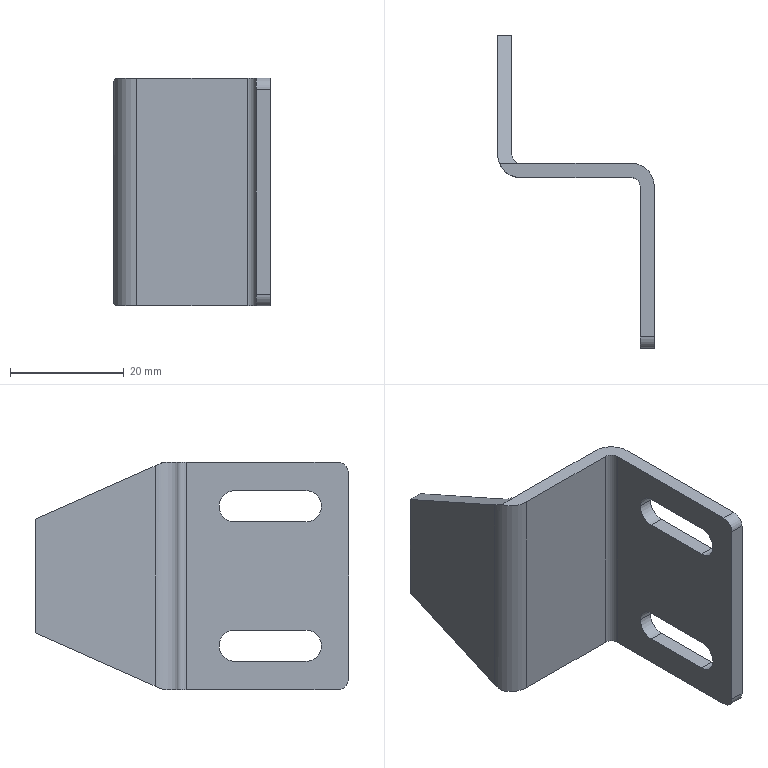Part | NX | features BREP 1 | 1 solid | 28 faces | box 27.5 x 55 x 40 mm | volume 6735 mm3 | plane 16 | cylinder 12 | commonest cylinder face diameters 5.5 x6 3 x2 4 x2 8 x2
STEP:
#1=CARTESIAN_POINT('',(0.,-7.25,-12.25));
#2=VERTEX_POINT('',#1);
#3=CARTESIAN_POINT('',(0.,-10.,-9.5));
#4=VERTEX_POINT('',#3);
#5=CARTESIAN_POINT('',(0.,-10.,-12.25));
#6=DIRECTION('',(1.,0.,0.));
#7=DIRECTION('',(0.,1.,0.));
#8=AXIS2_PLACEMENT_3D('',#5,#6,#7);
#9=CIRCLE('',#8,2.75);
#10=EDGE_CURVE('',#2,#4,#9,.T.);
#11=ORIENTED_EDGE('',*,*,#10,.F.);
#12=CARTESIAN_POINT('',(2.5,-7.25,-12.25));
#13=VERTEX_POINT('',#12);
#14=CARTESIAN_POINT('',(-25.,-7.25,-12.25));
#15=DIRECTION('',(1.,0.,0.));
#16=VECTOR('',#15,1000.);
#17=LINE('',#14,#16);
#18=EDGE_CURVE('',#2,#13,#17,.T.);
#19=ORIENTED_EDGE('',*,*,#18,.T.);
#20=CARTESIAN_POINT('',(2.5,-10.,-9.5));
#21=VERTEX_POINT('',#20);
#22=CARTESIAN_POINT('',(2.5,-10.,-12.25));
#23=DIRECTION('',(1.,0.,0.));
#24=DIRECTION('',(0.,-1.,0.));
#25=AXIS2_PLACEMENT_3D('',#22,#23,#24);
#26=CIRCLE('',#25,2.75);
#27=EDGE_CURVE('',#13,#21,#26,.T.);
#28=ORIENTED_EDGE('',*,*,#27,.T.);
#29=CARTESIAN_POINT('',(-25.,-10.,-9.5));
#30=DIRECTION('',(1.,0.,0.));
#31=VECTOR('',#30,1000.);
#32=LINE('',#29,#31);
#33=EDGE_CURVE('',#4,#21,#32,.T.);
#34=ORIENTED_EDGE('',*,*,#33,.F.);
#35=EDGE_LOOP('',(#11,#19,#28,#34));
#36=FACE_BOUND('',#35,.T.);
#37=CARTESIAN_POINT('',(-25.,-10.,-12.25));
#38=DIRECTION('',(1.,0.,0.));
#39=DIRECTION('',(0.,1.,0.));
#40=AXIS2_PLACEMENT_3D('',#37,#38,#39);
#41=CYLINDRICAL_SURFACE('',#40,2.75);
#42=ADVANCED_FACE('',(#36),#41,.F.);
#43=CARTESIAN_POINT('',(0.,-7.25,12.25));
#44=VERTEX_POINT('',#43);
#45=CARTESIAN_POINT('',(0.,-10.,15.));
#46=VERTEX_POINT('',#45);
#47=CARTESIAN_POINT('',(0.,-10.,12.25));
#48=DIRECTION('',(1.,0.,0.));
#49=DIRECTION('',(0.,1.,0.));
#50=AXIS2_PLACEMENT_3D('',#47,#48,#49);
#51=CIRCLE('',#50,2.75);
#52=EDGE_CURVE('',#44,#46,#51,.T.);
#53=ORIENTED_EDGE('',*,*,#52,.F.);
#54=CARTESIAN_POINT('',(2.5,-7.25,12.25));
#55=VERTEX_POINT('',#54);
#56=CARTESIAN_POINT('',(-25.,-7.25,12.25));
#57=DIRECTION('',(1.,0.,0.));
#58=VECTOR('',#57,1000.);
#59=LINE('',#56,#58);
#60=EDGE_CURVE('',#44,#55,#59,.T.);
#61=ORIENTED_EDGE('',*,*,#60,.T.);
#62=CARTESIAN_POINT('',(2.5,-10.,15.));
#63=VERTEX_POINT('',#62);
#64=CARTESIAN_POINT('',(2.5,-10.,12.25));
#65=DIRECTION('',(1.,0.,0.));
#66=DIRECTION('',(0.,1.,0.));
#67=AXIS2_PLACEMENT_3D('',#64,#65,#66);
#68=CIRCLE('',#67,2.75);
#69=EDGE_CURVE('',#55,#63,#68,.T.);
#70=ORIENTED_EDGE('',*,*,#69,.T.);
#71=CARTESIAN_POINT('',(-25.,-10.,15.));
#72=DIRECTION('',(1.,0.,0.));
#73=VECTOR('',#72,1000.);
#74=LINE('',#71,#73);
#75=EDGE_CURVE('',#46,#63,#74,.T.);
#76=ORIENTED_EDGE('',*,*,#75,.F.);
#77=EDGE_LOOP('',(#53,#61,#70,#76));
#78=FACE_BOUND('',#77,.T.);
#79=CARTESIAN_POINT('',(-25.,-10.,12.25));
#80=DIRECTION('',(1.,0.,0.));
#81=DIRECTION('',(0.,1.,0.));
#82=AXIS2_PLACEMENT_3D('',#79,#80,#81);
#83=CYLINDRICAL_SURFACE('',#82,2.75);
#84=ADVANCED_FACE('',(#78),#83,.F.);
#85=CARTESIAN_POINT('',(2.5,-30.,18.));
#86=VERTEX_POINT('',#85);
#87=CARTESIAN_POINT('',(2.5,-30.,-18.));
#88=VERTEX_POINT('',#87);
#89=CARTESIAN_POINT('',(2.5,-30.,20.));
#90=DIRECTION('',(0.,0.,-1.));
#91=VECTOR('',#90,1000.);
#92=LINE('',#89,#91);
#93=EDGE_CURVE('',#86,#88,#92,.T.);
#94=ORIENTED_EDGE('',*,*,#93,.T.);
#95=CARTESIAN_POINT('',(2.5,-28.,-20.));
#96=VERTEX_POINT('',#95);
#97=CARTESIAN_POINT('',(2.5,-28.,-18.));
#98=DIRECTION('',(1.,0.,0.));
#99=DIRECTION('',(0.,-1.,0.));
#100=AXIS2_PLACEMENT_3D('',#97,#98,#99);
#101=CIRCLE('',#100,2.);
#102=EDGE_CURVE('',#88,#96,#101,.T.);
#103=ORIENTED_EDGE('',*,*,#102,.T.);
#104=CARTESIAN_POINT('',(2.5,-1.5,-20.));
#105=VERTEX_POINT('',#104);
#106=CARTESIAN_POINT('',(2.5,2.5,-20.));
#107=DIRECTION('',(0.,1.,0.));
#108=VECTOR('',#107,1000.);
#109=LINE('',#106,#108);
#110=EDGE_CURVE('',#96,#105,#109,.T.);
#111=ORIENTED_EDGE('',*,*,#110,.T.);
#112=CARTESIAN_POINT('',(2.5,-1.5,20.));
#113=VERTEX_POINT('',#112);
#114=CARTESIAN_POINT('',(2.5,-1.5,20.));
#115=DIRECTION('',(0.,0.,1.));
#116=VECTOR('',#115,1000.);
#117=LINE('',#114,#116);
#118=EDGE_CURVE('',#105,#113,#117,.T.);
#119=ORIENTED_EDGE('',*,*,#118,.T.);
#120=CARTESIAN_POINT('',(2.5,-28.,20.));
#121=VERTEX_POINT('',#120);
#122=CARTESIAN_POINT('',(2.5,2.5,20.));
#123=DIRECTION('',(0.,1.,0.));
#124=VECTOR('',#123,1000.);
#125=LINE('',#122,#124);
#126=EDGE_CURVE('',#121,#113,#125,.T.);
#127=ORIENTED_EDGE('',*,*,#126,.F.);
#128=CARTESIAN_POINT('',(2.5,-28.,18.));
#129=DIRECTION('',(1.,0.,0.));
#130=DIRECTION('',(0.,-1.,0.));
#131=AXIS2_PLACEMENT_3D('',#128,#129,#130);
#132=CIRCLE('',#131,2.);
#133=EDGE_CURVE('',#121,#86,#132,.T.);
#134=ORIENTED_EDGE('',*,*,#133,.T.);
#135=EDGE_LOOP('',(#94,#103,#111,#119,#127,#134));
#136=FACE_BOUND('',#135,.T.);
#137=CARTESIAN_POINT('',(2.5,-22.5,-9.5));
#138=VERTEX_POINT('',#137);
#139=CARTESIAN_POINT('',(2.5,-10.,-9.5));
#140=DIRECTION('',(0.,-1.,0.));
#141=VECTOR('',#140,1000.);
#142=LINE('',#139,#141);
#143=EDGE_CURVE('',#21,#138,#142,.T.);
#144=ORIENTED_EDGE('',*,*,#143,.F.);
#145=ORIENTED_EDGE('',*,*,#27,.F.);
#146=CARTESIAN_POINT('',(2.5,-10.,-15.));
#147=VERTEX_POINT('',#146);
#148=CARTESIAN_POINT('',(2.5,-10.,-12.25));
#149=DIRECTION('',(1.,0.,0.));
#150=DIRECTION('',(0.,-1.,0.));
#151=AXIS2_PLACEMENT_3D('',#148,#149,#150);
#152=CIRCLE('',#151,2.75);
#153=EDGE_CURVE('',#147,#13,#152,.T.);
#154=ORIENTED_EDGE('',*,*,#153,.F.);
#155=CARTESIAN_POINT('',(2.5,-22.5,-15.));
#156=VERTEX_POINT('',#155);
#157=CARTESIAN_POINT('',(2.5,-10.,-15.));
#158=DIRECTION('',(0.,1.,0.));
#159=VECTOR('',#158,1000.);
#160=LINE('',#157,#159);
#161=EDGE_CURVE('',#156,#147,#160,.T.);
#162=ORIENTED_EDGE('',*,*,#161,.F.);
#163=CARTESIAN_POINT('',(2.5,-22.5,-12.25));
#164=DIRECTION('',(1.,0.,0.));
#165=DIRECTION('',(0.,-1.,0.));
#166=AXIS2_PLACEMENT_3D('',#163,#164,#165);
#167=CIRCLE('',#166,2.75);
#168=EDGE_CURVE('',#138,#156,#167,.T.);
#169=ORIENTED_EDGE('',*,*,#168,.F.);
#170=EDGE_LOOP('',(#144,#145,#154,#162,#169));
#171=FACE_BOUND('',#170,.T.);
#172=CARTESIAN_POINT('',(2.5,-22.5,15.));
#173=VERTEX_POINT('',#172);
#174=CARTESIAN_POINT('',(2.5,-10.,15.));
#175=DIRECTION('',(0.,-1.,0.));
#176=VECTOR('',#175,1000.);
#177=LINE('',#174,#176);
#178=EDGE_CURVE('',#63,#173,#177,.T.);
#179=ORIENTED_EDGE('',*,*,#178,.F.);
#180=ORIENTED_EDGE('',*,*,#69,.F.);
#181=CARTESIAN_POINT('',(2.5,-10.,9.5));
#182=VERTEX_POINT('',#181);
#183=CARTESIAN_POINT('',(2.5,-10.,12.25));
#184=DIRECTION('',(1.,0.,0.));
#185=DIRECTION('',(0.,1.,0.));
#186=AXIS2_PLACEMENT_3D('',#183,#184,#185);
#187=CIRCLE('',#186,2.75);
#188=EDGE_CURVE('',#182,#55,#187,.T.);
#189=ORIENTED_EDGE('',*,*,#188,.F.);
#190=CARTESIAN_POINT('',(2.5,-22.5,9.5));
#191=VERTEX_POINT('',#190);
#192=CARTESIAN_POINT('',(2.5,-10.,9.5));
#193=DIRECTION('',(0.,1.,0.));
#194=VECTOR('',#193,1000.);
#195=LINE('',#192,#194);
#196=EDGE_CURVE('',#191,#182,#195,.T.);
#197=ORIENTED_EDGE('',*,*,#196,.F.);
#198=CARTESIAN_POINT('',(2.5,-22.5,12.25));
#199=DIRECTION('',(1.,0.,0.));
#200=DIRECTION('',(0.,1.,0.));
#201=AXIS2_PLACEMENT_3D('',#198,#199,#200);
#202=CIRCLE('',#201,2.75);
#203=EDGE_CURVE('',#173,#191,#202,.T.);
#204=ORIENTED_EDGE('',*,*,#203,.F.);
#205=EDGE_LOOP('',(#179,#180,#189,#197,#204));
#206=FACE_BOUND('',#205,.T.);
#207=CARTESIAN_POINT('',(2.5,2.5,20.));
#208=DIRECTION('',(-1.,0.,0.));
#209=DIRECTION('',(0.,1.,0.));
#210=AXIS2_PLACEMENT_3D('',#207,#208,#209);
#211=PLANE('',#210);
#212=ADVANCED_FACE('',(#136,#171,#206),#211,.F.);
#213=CARTESIAN_POINT('',(-1.5,2.5,20.));
#214=VERTEX_POINT('',#213);
#215=CARTESIAN_POINT('',(-21.,2.5,20.));
#216=VERTEX_POINT('',#215);
#217=CARTESIAN_POINT('',(-22.5,2.5,20.));
#218=DIRECTION('',(-1.,0.,0.));
#219=VECTOR('',#218,1000.);
#220=LINE('',#217,#219);
#221=EDGE_CURVE('',#214,#216,#220,.T.);
#222=ORIENTED_EDGE('',*,*,#221,.F.);
#223=CARTESIAN_POINT('',(-1.5,2.5,-20.));
#224=VERTEX_POINT('',#223);
#225=CARTESIAN_POINT('',(-1.5,2.5,20.));
#226=DIRECTION('',(0.,0.,-1.));
#227=VECTOR('',#226,1000.);
#228=LINE('',#225,#227);
#229=EDGE_CURVE('',#214,#224,#228,.T.);
#230=ORIENTED_EDGE('',*,*,#229,.T.);
#231=CARTESIAN_POINT('',(-21.,2.5,-20.));
#232=VERTEX_POINT('',#231);
#233=CARTESIAN_POINT('',(-22.5,2.5,-20.));
#234=DIRECTION('',(-1.,0.,0.));
#235=VECTOR('',#234,1000.);
#236=LINE('',#233,#235);
#237=EDGE_CURVE('',#224,#232,#236,.T.);
#238=ORIENTED_EDGE('',*,*,#237,.T.);
#239=CARTESIAN_POINT('',(-21.,2.5,20.));
#240=DIRECTION('',(0.,0.,1.));
#241=VECTOR('',#240,1000.);
#242=LINE('',#239,#241);
#243=EDGE_CURVE('',#232,#216,#242,.T.);
#244=ORIENTED_EDGE('',*,*,#243,.T.);
#245=EDGE_LOOP('',(#222,#230,#238,#244));
#246=FACE_BOUND('',#245,.T.);
#247=CARTESIAN_POINT('',(-22.5,2.5,20.));
#248=DIRECTION('',(0.,-1.,0.));
#249=DIRECTION('',(0.,0.,-1.));
#250=AXIS2_PLACEMENT_3D('',#247,#248,#249);
#251=PLANE('',#250);
#252=ADVANCED_FACE('',(#246),#251,.F.);
#253=CARTESIAN_POINT('',(-22.5,25.,10.));
#254=VERTEX_POINT('',#253);
#255=CARTESIAN_POINT('',(-22.5,4.,19.333));
#256=VERTEX_POINT('',#255);
#257=CARTESIAN_POINT('',(-22.5,21.289,11.649));
#258=DIRECTION('',(0.,-0.9138,0.4061));
#259=VECTOR('',#258,1000.);
#260=LINE('',#257,#259);
#261=EDGE_CURVE('',#254,#256,#260,.T.);
#262=ORIENTED_EDGE('',*,*,#261,.T.);
#263=CARTESIAN_POINT('',(-22.5,4.,-19.333));
#264=VERTEX_POINT('',#263);
#265=CARTESIAN_POINT('',(-22.5,4.,-20.));
#266=DIRECTION('',(0.,0.,-1.));
#267=VECTOR('',#266,1000.);
#268=LINE('',#265,#267);
#269=EDGE_CURVE('',#256,#264,#268,.T.);
#270=ORIENTED_EDGE('',*,*,#269,.T.);
#271=CARTESIAN_POINT('',(-22.5,25.,-10.));
#272=VERTEX_POINT('',#271);
#273=CARTESIAN_POINT('',(-22.5,36.134,-5.052));
#274=DIRECTION('',(0.,0.9138,0.4061));
#275=VECTOR('',#274,1000.);
#276=LINE('',#273,#275);
#277=EDGE_CURVE('',#264,#272,#276,.T.);
#278=ORIENTED_EDGE('',*,*,#277,.T.);
#279=CARTESIAN_POINT('',(-22.5,25.,20.));
#280=DIRECTION('',(0.,0.,-1.));
#281=VECTOR('',#280,1000.);
#282=LINE('',#279,#281);
#283=EDGE_CURVE('',#254,#272,#282,.T.);
#284=ORIENTED_EDGE('',*,*,#283,.F.);
#285=EDGE_LOOP('',(#262,#270,#278,#284));
#286=FACE_BOUND('',#285,.T.);
#287=CARTESIAN_POINT('',(-22.5,25.,20.));
#288=DIRECTION('',(-1.,0.,0.));
#289=DIRECTION('',(0.,1.,0.));
#290=AXIS2_PLACEMENT_3D('',#287,#288,#289);
#291=PLANE('',#290);
#292=ADVANCED_FACE('',(#286),#291,.F.);
#293=ORIENTED_EDGE('',*,*,#283,.T.);
#294=CARTESIAN_POINT('',(-25.,25.,-10.));
#295=VERTEX_POINT('',#294);
#296=CARTESIAN_POINT('',(-25.,25.,-10.));
#297=DIRECTION('',(1.,0.,0.));
#298=VECTOR('',#297,1000.);
#299=LINE('',#296,#298);
#300=EDGE_CURVE('',#295,#272,#299,.T.);
#301=ORIENTED_EDGE('',*,*,#300,.F.);
#302=CARTESIAN_POINT('',(-25.,25.,10.));
#303=VERTEX_POINT('',#302);
#304=CARTESIAN_POINT('',(-25.,25.,20.));
#305=DIRECTION('',(0.,0.,-1.));
#306=VECTOR('',#305,1000.);
#307=LINE('',#304,#306);
#308=EDGE_CURVE('',#303,#295,#307,.T.);
#309=ORIENTED_EDGE('',*,*,#308,.F.);
#310=CARTESIAN_POINT('',(-25.,25.,10.));
#311=DIRECTION('',(1.,0.,0.));
#312=VECTOR('',#311,1000.);
#313=LINE('',#310,#312);
#314=EDGE_CURVE('',#303,#254,#313,.T.);
#315=ORIENTED_EDGE('',*,*,#314,.T.);
#316=EDGE_LOOP('',(#293,#301,#309,#315));
#317=FACE_BOUND('',#316,.T.);
#318=CARTESIAN_POINT('',(-25.,25.,20.));
#319=DIRECTION('',(0.,-1.,0.));
#320=DIRECTION('',(0.,0.,-1.));
#321=AXIS2_PLACEMENT_3D('',#318,#319,#320);
#322=PLANE('',#321);
#323=ADVANCED_FACE('',(#317),#322,.F.);
#324=CARTESIAN_POINT('',(-25.,4.,-19.333));
#325=VERTEX_POINT('',#324);
#326=CARTESIAN_POINT('',(-25.,25.,-10.));
#327=DIRECTION('',(0.,-0.9138,-0.4061));
#328=VECTOR('',#327,1000.);
#329=LINE('',#326,#328);
#330=EDGE_CURVE('',#295,#325,#329,.T.);
#331=ORIENTED_EDGE('',*,*,#330,.T.);
#332=CARTESIAN_POINT('',(-25.,4.,19.333));
#333=VERTEX_POINT('',#332);
#334=CARTESIAN_POINT('',(-25.,4.,20.));
#335=DIRECTION('',(0.,0.,1.));
#336=VECTOR('',#335,1000.);
#337=LINE('',#334,#336);
#338=EDGE_CURVE('',#325,#333,#337,.T.);
#339=ORIENTED_EDGE('',*,*,#338,.T.);
#340=CARTESIAN_POINT('',(-25.,25.,10.));
#341=DIRECTION('',(0.,0.9138,-0.4061));
#342=VECTOR('',#341,1000.);
#343=LINE('',#340,#342);
#344=EDGE_CURVE('',#333,#303,#343,.T.);
#345=ORIENTED_EDGE('',*,*,#344,.T.);
#346=ORIENTED_EDGE('',*,*,#308,.T.);
#347=EDGE_LOOP('',(#331,#339,#345,#346));
#348=FACE_BOUND('',#347,.T.);
#349=CARTESIAN_POINT('',(-25.,0.,20.));
#350=DIRECTION('',(1.,0.,0.));
#351=DIRECTION('',(0.,1.,0.));
#352=AXIS2_PLACEMENT_3D('',#349,#350,#351);
#353=PLANE('',#352);
#354=ADVANCED_FACE('',(#348),#353,.F.);
#355=CARTESIAN_POINT('',(-21.,0.,20.));
#356=VERTEX_POINT('',#355);
#357=CARTESIAN_POINT('',(-1.5,0.,20.));
#358=VERTEX_POINT('',#357);
#359=CARTESIAN_POINT('',(0.,0.,20.));
#360=DIRECTION('',(1.,0.,0.));
#361=VECTOR('',#360,1000.);
#362=LINE('',#359,#361);
#363=EDGE_CURVE('',#356,#358,#362,.T.);
#364=ORIENTED_EDGE('',*,*,#363,.F.);
#365=CARTESIAN_POINT('',(-21.,0.,-20.));
#366=VERTEX_POINT('',#365);
#367=CARTESIAN_POINT('',(-21.,0.,20.));
#368=DIRECTION('',(0.,0.,-1.));
#369=VECTOR('',#368,1000.);
#370=LINE('',#367,#369);
#371=EDGE_CURVE('',#356,#366,#370,.T.);
#372=ORIENTED_EDGE('',*,*,#371,.T.);
#373=CARTESIAN_POINT('',(-1.5,0.,-20.));
#374=VERTEX_POINT('',#373);
#375=CARTESIAN_POINT('',(0.,0.,-20.));
#376=DIRECTION('',(1.,0.,0.));
#377=VECTOR('',#376,1000.);
#378=LINE('',#375,#377);
#379=EDGE_CURVE('',#366,#374,#378,.T.);
#380=ORIENTED_EDGE('',*,*,#379,.T.);
#381=CARTESIAN_POINT('',(-1.5,0.,20.));
#382=DIRECTION('',(0.,0.,1.));
#383=VECTOR('',#382,1000.);
#384=LINE('',#381,#383);
#385=EDGE_CURVE('',#374,#358,#384,.T.);
#386=ORIENTED_EDGE('',*,*,#385,.T.);
#387=EDGE_LOOP('',(#364,#372,#380,#386));
#388=FACE_BOUND('',#387,.T.);
#389=CARTESIAN_POINT('',(0.,0.,20.));
#390=DIRECTION('',(0.,1.,0.));
#391=DIRECTION('',(1.,0.,0.));
#392=AXIS2_PLACEMENT_3D('',#389,#390,#391);
#393=PLANE('',#392);
#394=ADVANCED_FACE('',(#388),#393,.F.);
#395=CARTESIAN_POINT('',(0.,-1.5,-20.));
#396=VERTEX_POINT('',#395);
#397=CARTESIAN_POINT('',(0.,-28.,-20.));
#398=VERTEX_POINT('',#397);
#399=CARTESIAN_POINT('',(0.,-30.,-20.));
#400=DIRECTION('',(0.,-1.,0.));
#401=VECTOR('',#400,1000.);
#402=LINE('',#399,#401);
#403=EDGE_CURVE('',#396,#398,#402,.T.);
#404=ORIENTED_EDGE('',*,*,#403,.T.);
#405=CARTESIAN_POINT('',(0.,-30.,-18.));
#406=VERTEX_POINT('',#405);
#407=CARTESIAN_POINT('',(0.,-28.,-18.));
#408=DIRECTION('',(-1.,0.,0.));
#409=DIRECTION('',(0.,1.,0.));
#410=AXIS2_PLACEMENT_3D('',#407,#408,#409);
#411=CIRCLE('',#410,2.);
#412=EDGE_CURVE('',#398,#406,#411,.T.);
#413=ORIENTED_EDGE('',*,*,#412,.T.);
#414=CARTESIAN_POINT('',(0.,-30.,18.));
#415=VERTEX_POINT('',#414);
#416=CARTESIAN_POINT('',(0.,-30.,20.));
#417=DIRECTION('',(0.,0.,-1.));
#418=VECTOR('',#417,1000.);
#419=LINE('',#416,#418);
#420=EDGE_CURVE('',#415,#406,#419,.T.);
#421=ORIENTED_EDGE('',*,*,#420,.F.);
#422=CARTESIAN_POINT('',(0.,-28.,20.));
#423=VERTEX_POINT('',#422);
#424=CARTESIAN_POINT('',(0.,-28.,18.));
#425=DIRECTION('',(-1.,0.,0.));
#426=DIRECTION('',(0.,1.,0.));
#427=AXIS2_PLACEMENT_3D('',#424,#425,#426);
#428=CIRCLE('',#427,2.);
#429=EDGE_CURVE('',#415,#423,#428,.T.);
#430=ORIENTED_EDGE('',*,*,#429,.T.);
#431=CARTESIAN_POINT('',(0.,-1.5,20.));
#432=VERTEX_POINT('',#431);
#433=CARTESIAN_POINT('',(0.,-30.,20.));
#434=DIRECTION('',(0.,-1.,0.));
#435=VECTOR('',#434,1000.);
#436=LINE('',#433,#435);
#437=EDGE_CURVE('',#432,#423,#436,.T.);
#438=ORIENTED_EDGE('',*,*,#437,.F.);
#439=CARTESIAN_POINT('',(0.,-1.5,-20.));
#440=DIRECTION('',(0.,0.,-1.));
#441=VECTOR('',#440,1000.);
#442=LINE('',#439,#441);
#443=EDGE_CURVE('',#432,#396,#442,.T.);
#444=ORIENTED_EDGE('',*,*,#443,.T.);
#445=EDGE_LOOP('',(#404,#413,#421,#430,#438,#444));
#446=FACE_BOUND('',#445,.T.);
#447=CARTESIAN_POINT('',(0.,-22.5,-15.));
#448=VERTEX_POINT('',#447);
#449=CARTESIAN_POINT('',(0.,-10.,-15.));
#450=VERTEX_POINT('',#449);
#451=CARTESIAN_POINT('',(0.,-30.,-15.));
#452=DIRECTION('',(0.,1.,0.));
#453=VECTOR('',#452,1000.);
#454=LINE('',#451,#453);
#455=EDGE_CURVE('',#448,#450,#454,.T.);
#456=ORIENTED_EDGE('',*,*,#455,.T.);
#457=CARTESIAN_POINT('',(0.,-10.,-12.25));
#458=DIRECTION('',(1.,0.,0.));
#459=DIRECTION('',(0.,1.,0.));
#460=AXIS2_PLACEMENT_3D('',#457,#458,#459);
#461=CIRCLE('',#460,2.75);
#462=EDGE_CURVE('',#450,#2,#461,.T.);
#463=ORIENTED_EDGE('',*,*,#462,.T.);
#464=ORIENTED_EDGE('',*,*,#10,.T.);
#465=CARTESIAN_POINT('',(0.,-22.5,-9.5));
#466=VERTEX_POINT('',#465);
#467=CARTESIAN_POINT('',(0.,-30.,-9.5));
#468=DIRECTION('',(0.,-1.,0.));
#469=VECTOR('',#468,1000.);
#470=LINE('',#467,#469);
#471=EDGE_CURVE('',#4,#466,#470,.T.);
#472=ORIENTED_EDGE('',*,*,#471,.T.);
#473=CARTESIAN_POINT('',(0.,-22.5,-12.25));
#474=DIRECTION('',(1.,0.,0.));
#475=DIRECTION('',(0.,1.,0.));
#476=AXIS2_PLACEMENT_3D('',#473,#474,#475);
#477=CIRCLE('',#476,2.75);
#478=EDGE_CURVE('',#466,#448,#477,.T.);
#479=ORIENTED_EDGE('',*,*,#478,.T.);
#480=EDGE_LOOP('',(#456,#463,#464,#472,#479));
#481=FACE_BOUND('',#480,.T.);
#482=CARTESIAN_POINT('',(0.,-22.5,9.5));
#483=VERTEX_POINT('',#482);
#484=CARTESIAN_POINT('',(0.,-10.,9.5));
#485=VERTEX_POINT('',#484);
#486=CARTESIAN_POINT('',(0.,-30.,9.5));
#487=DIRECTION('',(0.,1.,0.));
#488=VECTOR('',#487,1000.);
#489=LINE('',#486,#488);
#490=EDGE_CURVE('',#483,#485,#489,.T.);
#491=ORIENTED_EDGE('',*,*,#490,.T.);
#492=CARTESIAN_POINT('',(0.,-10.,12.25));
#493=DIRECTION('',(1.,0.,0.));
#494=DIRECTION('',(0.,1.,0.));
#495=AXIS2_PLACEMENT_3D('',#492,#493,#494);
#496=CIRCLE('',#495,2.75);
#497=EDGE_CURVE('',#485,#44,#496,.T.);
#498=ORIENTED_EDGE('',*,*,#497,.T.);
#499=ORIENTED_EDGE('',*,*,#52,.T.);
#500=CARTESIAN_POINT('',(0.,-22.5,15.));
#501=VERTEX_POINT('',#500);
#502=CARTESIAN_POINT('',(0.,-30.,15.));
#503=DIRECTION('',(0.,-1.,0.));
#504=VECTOR('',#503,1000.);
#505=LINE('',#502,#504);
#506=EDGE_CURVE('',#46,#501,#505,.T.);
#507=ORIENTED_EDGE('',*,*,#506,.T.);
#508=CARTESIAN_POINT('',(0.,-22.5,12.25));
#509=DIRECTION('',(1.,0.,0.));
#510=DIRECTION('',(0.,1.,0.));
#511=AXIS2_PLACEMENT_3D('',#508,#509,#510);
#512=CIRCLE('',#511,2.75);
#513=EDGE_CURVE('',#501,#483,#512,.T.);
#514=ORIENTED_EDGE('',*,*,#513,.T.);
#515=EDGE_LOOP('',(#491,#498,#499,#507,#514));
#516=FACE_BOUND('',#515,.T.);
#517=CARTESIAN_POINT('',(0.,-30.,20.));
#518=DIRECTION('',(1.,0.,0.));
#519=DIRECTION('',(0.,1.,0.));
#520=AXIS2_PLACEMENT_3D('',#517,#518,#519);
#521=PLANE('',#520);
#522=ADVANCED_FACE('',(#446,#481,#516),#521,.F.);
#523=ORIENTED_EDGE('',*,*,#420,.T.);
#524=CARTESIAN_POINT('',(2.5,-30.,-18.));
#525=DIRECTION('',(1.,0.,0.));
#526=VECTOR('',#525,1000.);
#527=LINE('',#524,#526);
#528=EDGE_CURVE('',#406,#88,#527,.T.);
#529=ORIENTED_EDGE('',*,*,#528,.T.);
#530=ORIENTED_EDGE('',*,*,#93,.F.);
#531=CARTESIAN_POINT('',(2.5,-30.,18.));
#532=DIRECTION('',(-1.,0.,0.));
#533=VECTOR('',#532,1000.);
#534=LINE('',#531,#533);
#535=EDGE_CURVE('',#86,#415,#534,.T.);
#536=ORIENTED_EDGE('',*,*,#535,.T.);
#537=EDGE_LOOP('',(#523,#529,#530,#536));
#538=FACE_BOUND('',#537,.T.);
#539=CARTESIAN_POINT('',(2.5,-30.,20.));
#540=DIRECTION('',(0.,1.,0.));
#541=DIRECTION('',(1.,0.,0.));
#542=AXIS2_PLACEMENT_3D('',#539,#540,#541);
#543=PLANE('',#542);
#544=ADVANCED_FACE('',(#538),#543,.F.);
#545=ORIENTED_EDGE('',*,*,#437,.T.);
#546=CARTESIAN_POINT('',(0.,-28.,20.));
#547=DIRECTION('',(1.,0.,0.));
#548=VECTOR('',#547,1000.);
#549=LINE('',#546,#548);
#550=EDGE_CURVE('',#423,#121,#549,.T.);
#551=ORIENTED_EDGE('',*,*,#550,.T.);
#552=ORIENTED_EDGE('',*,*,#126,.T.);
#553=CARTESIAN_POINT('',(-1.5,-1.5,20.));
#554=DIRECTION('',(0.,0.,1.));
#555=DIRECTION('',(-1.,0.,0.));
#556=AXIS2_PLACEMENT_3D('',#553,#554,#555);
#557=CIRCLE('',#556,4.);
#558=EDGE_CURVE('',#113,#214,#557,.T.);
#559=ORIENTED_EDGE('',*,*,#558,.T.);
#560=ORIENTED_EDGE('',*,*,#221,.T.);
#561=CARTESIAN_POINT('',(-24.708,2.5,20.));
#562=VERTEX_POINT('',#561);
#563=CARTESIAN_POINT('',(-25.,2.5,20.));
#564=DIRECTION('',(1.,0.,0.));
#565=VECTOR('',#564,1000.);
#566=LINE('',#563,#565);
#567=EDGE_CURVE('',#562,#216,#566,.T.);
#568=ORIENTED_EDGE('',*,*,#567,.F.);
#569=CARTESIAN_POINT('',(-21.,4.,20.));
#570=DIRECTION('',(0.,0.,1.));
#571=DIRECTION('',(-1.,0.,0.));
#572=AXIS2_PLACEMENT_3D('',#569,#570,#571);
#573=CIRCLE('',#572,4.);
#574=EDGE_CURVE('',#562,#356,#573,.T.);
#575=ORIENTED_EDGE('',*,*,#574,.T.);
#576=ORIENTED_EDGE('',*,*,#363,.T.);
#577=CARTESIAN_POINT('',(-1.5,-1.5,20.));
#578=DIRECTION('',(0.,0.,-1.));
#579=DIRECTION('',(-1.,0.,0.));
#580=AXIS2_PLACEMENT_3D('',#577,#578,#579);
#581=CIRCLE('',#580,1.5);
#582=EDGE_CURVE('',#358,#432,#581,.T.);
#583=ORIENTED_EDGE('',*,*,#582,.T.);
#584=EDGE_LOOP('',(#545,#551,#552,#559,#560,#568,#575,#576,#583));
#585=FACE_BOUND('',#584,.T.);
#586=CARTESIAN_POINT('',(0.,0.,20.));
#587=DIRECTION('',(0.,0.,-1.));
#588=DIRECTION('',(0.,-1.,0.));
#589=AXIS2_PLACEMENT_3D('',#586,#587,#588);
#590=PLANE('',#589);
#591=ADVANCED_FACE('',(#585),#590,.F.);
#592=ORIENTED_EDGE('',*,*,#110,.F.);
#593=CARTESIAN_POINT('',(0.,-28.,-20.));
#594=DIRECTION('',(-1.,0.,0.));
#595=VECTOR('',#594,1000.);
#596=LINE('',#593,#595);
#597=EDGE_CURVE('',#96,#398,#596,.T.);
#598=ORIENTED_EDGE('',*,*,#597,.T.);
#599=ORIENTED_EDGE('',*,*,#403,.F.);
#600=CARTESIAN_POINT('',(-1.5,-1.5,-20.));
#601=DIRECTION('',(0.,0.,1.));
#602=DIRECTION('',(-1.,0.,0.));
#603=AXIS2_PLACEMENT_3D('',#600,#601,#602);
#604=CIRCLE('',#603,1.5);
#605=EDGE_CURVE('',#396,#374,#604,.T.);
#606=ORIENTED_EDGE('',*,*,#605,.T.);
#607=ORIENTED_EDGE('',*,*,#379,.F.);
#608=CARTESIAN_POINT('',(-24.708,2.5,-20.));
#609=VERTEX_POINT('',#608);
#610=CARTESIAN_POINT('',(-21.,4.,-20.));
#611=DIRECTION('',(0.,0.,-1.));
#612=DIRECTION('',(-1.,0.,0.));
#613=AXIS2_PLACEMENT_3D('',#610,#611,#612);
#614=CIRCLE('',#613,4.);
#615=EDGE_CURVE('',#366,#609,#614,.T.);
#616=ORIENTED_EDGE('',*,*,#615,.T.);
#617=CARTESIAN_POINT('',(-25.,2.5,-20.));
#618=DIRECTION('',(1.,0.,0.));
#619=VECTOR('',#618,1000.);
#620=LINE('',#617,#619);
#621=EDGE_CURVE('',#609,#232,#620,.T.);
#622=ORIENTED_EDGE('',*,*,#621,.T.);
#623=ORIENTED_EDGE('',*,*,#237,.F.);
#624=CARTESIAN_POINT('',(-1.5,-1.5,-20.));
#625=DIRECTION('',(0.,0.,-1.));
#626=DIRECTION('',(-1.,0.,0.));
#627=AXIS2_PLACEMENT_3D('',#624,#625,#626);
#628=CIRCLE('',#627,4.);
#629=EDGE_CURVE('',#224,#105,#628,.T.);
#630=ORIENTED_EDGE('',*,*,#629,.T.);
#631=EDGE_LOOP('',(#592,#598,#599,#606,#607,#616,#622,#623,#630));
#632=FACE_BOUND('',#631,.T.);
#633=CARTESIAN_POINT('',(0.,0.,-20.));
#634=DIRECTION('',(0.,0.,-1.));
#635=DIRECTION('',(0.,-1.,0.));
#636=AXIS2_PLACEMENT_3D('',#633,#634,#635);
#637=PLANE('',#636);
#638=ADVANCED_FACE('',(#632),#637,.T.);
#639=ORIENTED_EDGE('',*,*,#344,.F.);
#640=CARTESIAN_POINT('',(-25.,4.,19.333));
#641=CARTESIAN_POINT('',(-25.,3.484,19.563));
#642=CARTESIAN_POINT('',(-24.901,2.978,19.788));
#643=CARTESIAN_POINT('',(-24.708,2.5,20.));
#644=(BOUNDED_CURVE()B_SPLINE_CURVE(3,(#640,#641,#642,#643),.UNSPECIFIED.,.F.,.F.)B_SPLINE_CURVE_WITH_KNOTS((4,4),(1.571,1.955),.UNSPECIFIED.)CURVE()GEOMETRIC_REPRESENTATION_ITEM()RATIONAL_B_SPLINE_CURVE((1.,0.9877,0.9877,1.))REPRESENTATION_ITEM(''));
#645=EDGE_CURVE('',#333,#562,#644,.T.);
#646=ORIENTED_EDGE('',*,*,#645,.T.);
#647=ORIENTED_EDGE('',*,*,#567,.T.);
#648=CARTESIAN_POINT('',(-21.,2.5,20.));
#649=CARTESIAN_POINT('',(-21.879,2.5,20.));
#650=CARTESIAN_POINT('',(-22.5,3.121,19.724));
#651=CARTESIAN_POINT('',(-22.5,4.,19.333));
#652=(BOUNDED_CURVE()B_SPLINE_CURVE(3,(#648,#649,#650,#651),.UNSPECIFIED.,.F.,.F.)B_SPLINE_CURVE_WITH_KNOTS((4,4),(0.,1.571),.UNSPECIFIED.)CURVE()GEOMETRIC_REPRESENTATION_ITEM()RATIONAL_B_SPLINE_CURVE((1.,0.8047,0.8047,1.))REPRESENTATION_ITEM(''));
#653=EDGE_CURVE('',#216,#256,#652,.T.);
#654=ORIENTED_EDGE('',*,*,#653,.T.);
#655=ORIENTED_EDGE('',*,*,#261,.F.);
#656=ORIENTED_EDGE('',*,*,#314,.F.);
#657=EDGE_LOOP('',(#639,#646,#647,#654,#655,#656));
#658=FACE_BOUND('',#657,.T.);
#659=CARTESIAN_POINT('',(-25.,25.,10.));
#660=DIRECTION('',(0.,-0.4061,-0.9138));
#661=DIRECTION('',(0.,-0.9138,0.4061));
#662=AXIS2_PLACEMENT_3D('',#659,#660,#661);
#663=PLANE('',#662);
#664=ADVANCED_FACE('',(#658),#663,.F.);
#665=ORIENTED_EDGE('',*,*,#621,.F.);
#666=CARTESIAN_POINT('',(-24.708,2.5,-20.));
#667=CARTESIAN_POINT('',(-24.901,2.978,-19.788));
#668=CARTESIAN_POINT('',(-25.,3.484,-19.563));
#669=CARTESIAN_POINT('',(-25.,4.,-19.333));
#670=(BOUNDED_CURVE()B_SPLINE_CURVE(3,(#666,#667,#668,#669),.UNSPECIFIED.,.F.,.F.)B_SPLINE_CURVE_WITH_KNOTS((4,4),(1.186,1.571),.UNSPECIFIED.)CURVE()GEOMETRIC_REPRESENTATION_ITEM()RATIONAL_B_SPLINE_CURVE((1.,0.9877,0.9877,1.))REPRESENTATION_ITEM(''));
#671=EDGE_CURVE('',#609,#325,#670,.T.);
#672=ORIENTED_EDGE('',*,*,#671,.T.);
#673=ORIENTED_EDGE('',*,*,#330,.F.);
#674=ORIENTED_EDGE('',*,*,#300,.T.);
#675=ORIENTED_EDGE('',*,*,#277,.F.);
#676=CARTESIAN_POINT('',(-22.5,4.,-19.333));
#677=CARTESIAN_POINT('',(-22.5,3.121,-19.724));
#678=CARTESIAN_POINT('',(-21.879,2.5,-20.));
#679=CARTESIAN_POINT('',(-21.,2.5,-20.));
#680=(BOUNDED_CURVE()B_SPLINE_CURVE(3,(#676,#677,#678,#679),.UNSPECIFIED.,.F.,.F.)B_SPLINE_CURVE_WITH_KNOTS((4,4),(1.571,3.142),.UNSPECIFIED.)CURVE()GEOMETRIC_REPRESENTATION_ITEM()RATIONAL_B_SPLINE_CURVE((1.,0.8047,0.8047,1.))REPRESENTATION_ITEM(''));
#681=EDGE_CURVE('',#264,#232,#680,.T.);
#682=ORIENTED_EDGE('',*,*,#681,.T.);
#683=EDGE_LOOP('',(#665,#672,#673,#674,#675,#682));
#684=FACE_BOUND('',#683,.T.);
#685=CARTESIAN_POINT('',(-25.,25.,-10.));
#686=DIRECTION('',(0.,-0.4061,0.9138));
#687=DIRECTION('',(-1.,0.,0.));
#688=AXIS2_PLACEMENT_3D('',#685,#686,#687);
#689=PLANE('',#688);
#690=ADVANCED_FACE('',(#684),#689,.F.);
#691=ORIENTED_EDGE('',*,*,#60,.F.);
#692=ORIENTED_EDGE('',*,*,#497,.F.);
#693=CARTESIAN_POINT('',(-25.,-10.,9.5));
#694=DIRECTION('',(1.,0.,0.));
#695=VECTOR('',#694,1000.);
#696=LINE('',#693,#695);
#697=EDGE_CURVE('',#485,#182,#696,.T.);
#698=ORIENTED_EDGE('',*,*,#697,.T.);
#699=ORIENTED_EDGE('',*,*,#188,.T.);
#700=EDGE_LOOP('',(#691,#692,#698,#699));
#701=FACE_BOUND('',#700,.T.);
#702=CARTESIAN_POINT('',(-25.,-10.,12.25));
#703=DIRECTION('',(1.,0.,0.));
#704=DIRECTION('',(0.,1.,0.));
#705=AXIS2_PLACEMENT_3D('',#702,#703,#704);
#706=CYLINDRICAL_SURFACE('',#705,2.75);
#707=ADVANCED_FACE('',(#701),#706,.F.);
#708=CARTESIAN_POINT('',(-25.,-22.5,9.5));
#709=DIRECTION('',(1.,0.,0.));
#710=VECTOR('',#709,1000.);
#711=LINE('',#708,#710);
#712=EDGE_CURVE('',#483,#191,#711,.T.);
#713=ORIENTED_EDGE('',*,*,#712,.T.);
#714=ORIENTED_EDGE('',*,*,#196,.T.);
#715=ORIENTED_EDGE('',*,*,#697,.F.);
#716=ORIENTED_EDGE('',*,*,#490,.F.);
#717=EDGE_LOOP('',(#713,#714,#715,#716));
#718=FACE_BOUND('',#717,.T.);
#719=CARTESIAN_POINT('',(-25.,-10.,9.5));
#720=DIRECTION('',(0.,0.,-1.));
#721=DIRECTION('',(-1.,0.,0.));
#722=AXIS2_PLACEMENT_3D('',#719,#720,#721);
#723=PLANE('',#722);
#724=ADVANCED_FACE('',(#718),#723,.F.);
#725=CARTESIAN_POINT('',(-25.,-22.5,15.));
#726=DIRECTION('',(1.,0.,0.));
#727=VECTOR('',#726,1000.);
#728=LINE('',#725,#727);
#729=EDGE_CURVE('',#501,#173,#728,.T.);
#730=ORIENTED_EDGE('',*,*,#729,.T.);
#731=ORIENTED_EDGE('',*,*,#203,.T.);
#732=ORIENTED_EDGE('',*,*,#712,.F.);
#733=ORIENTED_EDGE('',*,*,#513,.F.);
#734=EDGE_LOOP('',(#730,#731,#732,#733));
#735=FACE_BOUND('',#734,.T.);
#736=CARTESIAN_POINT('',(-25.,-22.5,12.25));
#737=DIRECTION('',(1.,0.,0.));
#738=DIRECTION('',(0.,1.,0.));
#739=AXIS2_PLACEMENT_3D('',#736,#737,#738);
#740=CYLINDRICAL_SURFACE('',#739,2.75);
#741=ADVANCED_FACE('',(#735),#740,.F.);
#742=ORIENTED_EDGE('',*,*,#75,.T.);
#743=ORIENTED_EDGE('',*,*,#178,.T.);
#744=ORIENTED_EDGE('',*,*,#729,.F.);
#745=ORIENTED_EDGE('',*,*,#506,.F.);
#746=EDGE_LOOP('',(#742,#743,#744,#745));
#747=FACE_BOUND('',#746,.T.);
#748=CARTESIAN_POINT('',(-25.,-10.,15.));
#749=DIRECTION('',(0.,0.,1.));
#750=DIRECTION('',(1.,0.,0.));
#751=AXIS2_PLACEMENT_3D('',#748,#749,#750);
#752=PLANE('',#751);
#753=ADVANCED_FACE('',(#747),#752,.F.);
#754=ORIENTED_EDGE('',*,*,#18,.F.);
#755=ORIENTED_EDGE('',*,*,#462,.F.);
#756=CARTESIAN_POINT('',(-25.,-10.,-15.));
#757=DIRECTION('',(1.,0.,0.));
#758=VECTOR('',#757,1000.);
#759=LINE('',#756,#758);
#760=EDGE_CURVE('',#450,#147,#759,.T.);
#761=ORIENTED_EDGE('',*,*,#760,.T.);
#762=ORIENTED_EDGE('',*,*,#153,.T.);
#763=EDGE_LOOP('',(#754,#755,#761,#762));
#764=FACE_BOUND('',#763,.T.);
#765=CARTESIAN_POINT('',(-25.,-10.,-12.25));
#766=DIRECTION('',(1.,0.,0.));
#767=DIRECTION('',(0.,1.,0.));
#768=AXIS2_PLACEMENT_3D('',#765,#766,#767);
#769=CYLINDRICAL_SURFACE('',#768,2.75);
#770=ADVANCED_FACE('',(#764),#769,.F.);
#771=CARTESIAN_POINT('',(-25.,-22.5,-15.));
#772=DIRECTION('',(1.,0.,0.));
#773=VECTOR('',#772,1000.);
#774=LINE('',#771,#773);
#775=EDGE_CURVE('',#448,#156,#774,.T.);
#776=ORIENTED_EDGE('',*,*,#775,.T.);
#777=ORIENTED_EDGE('',*,*,#161,.T.);
#778=ORIENTED_EDGE('',*,*,#760,.F.);
#779=ORIENTED_EDGE('',*,*,#455,.F.);
#780=EDGE_LOOP('',(#776,#777,#778,#779));
#781=FACE_BOUND('',#780,.T.);
#782=CARTESIAN_POINT('',(-25.,-10.,-15.));
#783=DIRECTION('',(0.,0.,-1.));
#784=DIRECTION('',(0.,-1.,0.));
#785=AXIS2_PLACEMENT_3D('',#782,#783,#784);
#786=PLANE('',#785);
#787=ADVANCED_FACE('',(#781),#786,.F.);
#788=CARTESIAN_POINT('',(-25.,-22.5,-9.5));
#789=DIRECTION('',(1.,0.,0.));
#790=VECTOR('',#789,1000.);
#791=LINE('',#788,#790);
#792=EDGE_CURVE('',#466,#138,#791,.T.);
#793=ORIENTED_EDGE('',*,*,#792,.T.);
#794=ORIENTED_EDGE('',*,*,#168,.T.);
#795=ORIENTED_EDGE('',*,*,#775,.F.);
#796=ORIENTED_EDGE('',*,*,#478,.F.);
#797=EDGE_LOOP('',(#793,#794,#795,#796));
#798=FACE_BOUND('',#797,.T.);
#799=CARTESIAN_POINT('',(-25.,-22.5,-12.25));
#800=DIRECTION('',(1.,0.,0.));
#801=DIRECTION('',(0.,1.,0.));
#802=AXIS2_PLACEMENT_3D('',#799,#800,#801);
#803=CYLINDRICAL_SURFACE('',#802,2.75);
#804=ADVANCED_FACE('',(#798),#803,.F.);
#805=ORIENTED_EDGE('',*,*,#33,.T.);
#806=ORIENTED_EDGE('',*,*,#143,.T.);
#807=ORIENTED_EDGE('',*,*,#792,.F.);
#808=ORIENTED_EDGE('',*,*,#471,.F.);
#809=EDGE_LOOP('',(#805,#806,#807,#808));
#810=FACE_BOUND('',#809,.T.);
#811=CARTESIAN_POINT('',(-25.,-10.,-9.5));
#812=DIRECTION('',(0.,0.,1.));
#813=DIRECTION('',(0.,-1.,0.));
#814=AXIS2_PLACEMENT_3D('',#811,#812,#813);
#815=PLANE('',#814);
#816=ADVANCED_FACE('',(#810),#815,.F.);
#817=ORIENTED_EDGE('',*,*,#412,.F.);
#818=ORIENTED_EDGE('',*,*,#597,.F.);
#819=ORIENTED_EDGE('',*,*,#102,.F.);
#820=ORIENTED_EDGE('',*,*,#528,.F.);
#821=EDGE_LOOP('',(#817,#818,#819,#820));
#822=FACE_BOUND('',#821,.T.);
#823=CARTESIAN_POINT('',(2.5,-28.,-18.));
#824=DIRECTION('',(-1.,0.,0.));
#825=DIRECTION('',(0.,0.,1.));
#826=AXIS2_PLACEMENT_3D('',#823,#824,#825);
#827=CYLINDRICAL_SURFACE('',#826,2.);
#828=ADVANCED_FACE('',(#822),#827,.T.);
#829=ORIENTED_EDGE('',*,*,#429,.F.);
#830=ORIENTED_EDGE('',*,*,#535,.F.);
#831=ORIENTED_EDGE('',*,*,#133,.F.);
#832=ORIENTED_EDGE('',*,*,#550,.F.);
#833=EDGE_LOOP('',(#829,#830,#831,#832));
#834=FACE_BOUND('',#833,.T.);
#835=CARTESIAN_POINT('',(0.,-28.,18.));
#836=DIRECTION('',(1.,0.,0.));
#837=DIRECTION('',(0.,0.,-1.));
#838=AXIS2_PLACEMENT_3D('',#835,#836,#837);
#839=CYLINDRICAL_SURFACE('',#838,2.);
#840=ADVANCED_FACE('',(#834),#839,.T.);
#841=ORIENTED_EDGE('',*,*,#645,.F.);
#842=ORIENTED_EDGE('',*,*,#338,.F.);
#843=ORIENTED_EDGE('',*,*,#671,.F.);
#844=ORIENTED_EDGE('',*,*,#615,.F.);
#845=ORIENTED_EDGE('',*,*,#371,.F.);
#846=ORIENTED_EDGE('',*,*,#574,.F.);
#847=EDGE_LOOP('',(#841,#842,#843,#844,#845,#846));
#848=FACE_BOUND('',#847,.T.);
#849=CARTESIAN_POINT('',(-21.,4.,20.));
#850=DIRECTION('',(0.,0.,-1.));
#851=DIRECTION('',(-1.,0.,0.));
#852=AXIS2_PLACEMENT_3D('',#849,#850,#851);
#853=CYLINDRICAL_SURFACE('',#852,4.);
#854=ADVANCED_FACE('',(#848),#853,.T.);
#855=ORIENTED_EDGE('',*,*,#558,.F.);
#856=ORIENTED_EDGE('',*,*,#118,.F.);
#857=ORIENTED_EDGE('',*,*,#629,.F.);
#858=ORIENTED_EDGE('',*,*,#229,.F.);
#859=EDGE_LOOP('',(#855,#856,#857,#858));
#860=FACE_BOUND('',#859,.T.);
#861=CARTESIAN_POINT('',(-1.5,-1.5,20.));
#862=DIRECTION('',(0.,0.,-1.));
#863=DIRECTION('',(-1.,0.,0.));
#864=AXIS2_PLACEMENT_3D('',#861,#862,#863);
#865=CYLINDRICAL_SURFACE('',#864,4.);
#866=ADVANCED_FACE('',(#860),#865,.T.);
#867=ORIENTED_EDGE('',*,*,#653,.F.);
#868=ORIENTED_EDGE('',*,*,#243,.F.);
#869=ORIENTED_EDGE('',*,*,#681,.F.);
#870=ORIENTED_EDGE('',*,*,#269,.F.);
#871=EDGE_LOOP('',(#867,#868,#869,#870));
#872=FACE_BOUND('',#871,.T.);
#873=CARTESIAN_POINT('',(-21.,4.,20.));
#874=DIRECTION('',(0.,0.,1.));
#875=DIRECTION('',(1.,0.,0.));
#876=AXIS2_PLACEMENT_3D('',#873,#874,#875);
#877=CYLINDRICAL_SURFACE('',#876,1.5);
#878=ADVANCED_FACE('',(#872),#877,.F.);
#879=ORIENTED_EDGE('',*,*,#582,.F.);
#880=ORIENTED_EDGE('',*,*,#385,.F.);
#881=ORIENTED_EDGE('',*,*,#605,.F.);
#882=ORIENTED_EDGE('',*,*,#443,.F.);
#883=EDGE_LOOP('',(#879,#880,#881,#882));
#884=FACE_BOUND('',#883,.T.);
#885=CARTESIAN_POINT('',(-1.5,-1.5,20.));
#886=DIRECTION('',(0.,0.,1.));
#887=DIRECTION('',(1.,0.,0.));
#888=AXIS2_PLACEMENT_3D('',#885,#886,#887);
#889=CYLINDRICAL_SURFACE('',#888,1.5);
#890=ADVANCED_FACE('',(#884),#889,.F.);
#891=CLOSED_SHELL('',(#42,#84,#212,#252,#292,#323,#354,#394,#522,#544,#591,#638,#664,#690,#707,#724,#741,#753,#770,#787,#804,#816,#828,#840,#854,#866,#878,#890));
#892=MANIFOLD_SOLID_BREP('',#891);
#893=(LENGTH_UNIT()NAMED_UNIT(*)SI_UNIT(.MILLI.,.METRE.));
#894=UNCERTAINTY_MEASURE_WITH_UNIT(LENGTH_MEASURE(0.00001),#893,'','');
#895=(NAMED_UNIT(*)PLANE_ANGLE_UNIT()SI_UNIT($,.RADIAN.));
#896=(NAMED_UNIT(*)SI_UNIT($,.STERADIAN.)SOLID_ANGLE_UNIT());
#897=(GEOMETRIC_REPRESENTATION_CONTEXT(3)GLOBAL_UNCERTAINTY_ASSIGNED_CONTEXT((#894))GLOBAL_UNIT_ASSIGNED_CONTEXT((#893,#895,#896))REPRESENTATION_CONTEXT('',''));
#898=ADVANCED_BREP_SHAPE_REPRESENTATION('',(#892),#897);